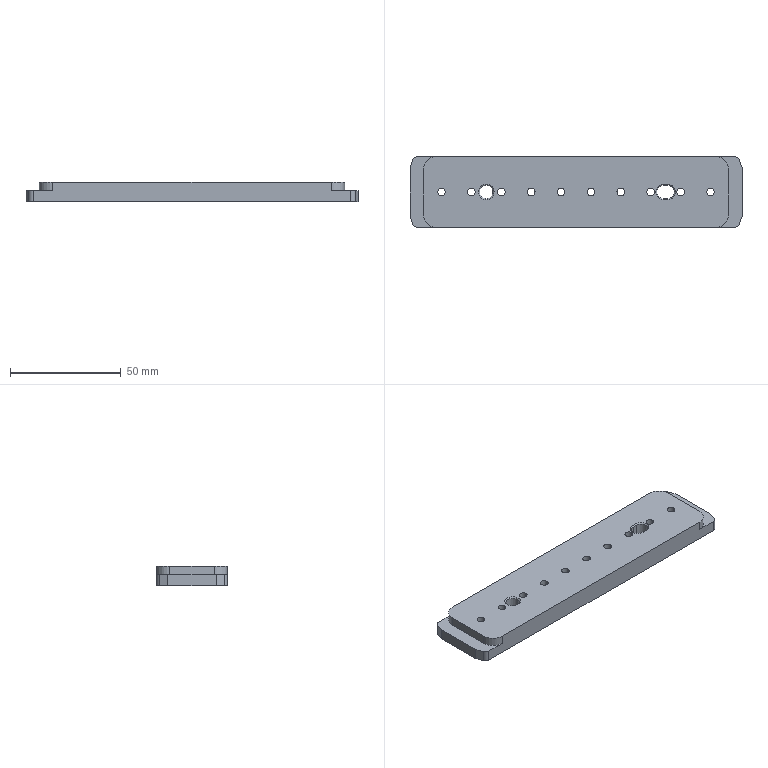Part | STEP file | QA-FB01 | 1 solid | 63 faces | box 150 x 32 x 9 mm | volume 39944 mm3 | cylinder 35 | plane 18 | cone 5 | torus 5 | commonest cylinder face diameters 3.5 x20 6 x5 4 x4 12 x4 2 x2